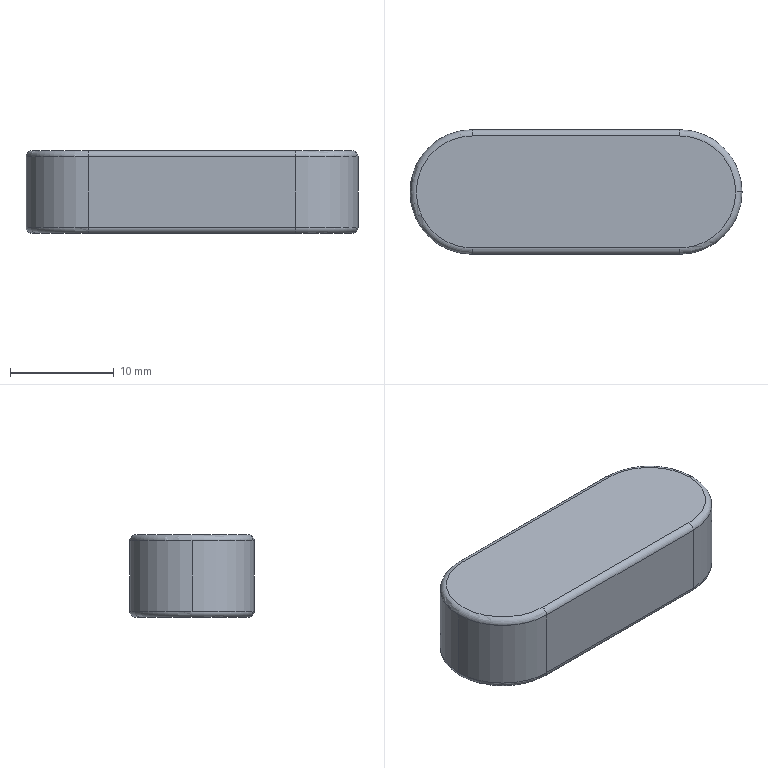Part | SolidWorks | features Extrusion 1, Fillet 1 | 1 solid | 17 faces | box 32 x 12 x 8 mm | volume 2813 mm3 | cylinder 7 | torus 6 | plane 4 | commonest cylinder face diameters 1.2 x4 12 x3
STEP:
#1=CARTESIAN_POINT('',(15.4,0.,0.));
#2=VERTEX_POINT('',#1);
#3=CARTESIAN_POINT('',(10.,-5.4,0.));
#4=VERTEX_POINT('',#3);
#5=CARTESIAN_POINT('',(10.,0.,0.));
#6=DIRECTION('',(0.,0.,-1.));
#7=DIRECTION('',(1.,0.,0.));
#8=AXIS2_PLACEMENT_3D('',#5,#6,#7);
#9=CIRCLE('',#8,5.4);
#10=EDGE_CURVE('',#2,#4,#9,.T.);
#11=ORIENTED_EDGE('',*,*,#10,.F.);
#12=CARTESIAN_POINT('',(16.,0.,0.6));
#13=VERTEX_POINT('',#12);
#14=CARTESIAN_POINT('',(15.4,0.,0.6));
#15=DIRECTION('',(0.,-1.,0.));
#16=DIRECTION('',(0.,0.,-1.));
#17=AXIS2_PLACEMENT_3D('',#14,#15,#16);
#18=CIRCLE('',#17,0.6);
#19=EDGE_CURVE('',#2,#13,#18,.T.);
#20=ORIENTED_EDGE('',*,*,#19,.T.);
#21=CARTESIAN_POINT('',(10.,-6.,0.6));
#22=VERTEX_POINT('',#21);
#23=CARTESIAN_POINT('',(10.,0.,0.6));
#24=DIRECTION('',(0.,0.,1.));
#25=DIRECTION('',(1.,0.,0.));
#26=AXIS2_PLACEMENT_3D('',#23,#24,#25);
#27=CIRCLE('',#26,6.);
#28=EDGE_CURVE('',#22,#13,#27,.T.);
#29=ORIENTED_EDGE('',*,*,#28,.F.);
#30=CARTESIAN_POINT('',(10.,-5.4,0.6));
#31=DIRECTION('',(1.,0.,0.));
#32=DIRECTION('',(0.,0.,-1.));
#33=AXIS2_PLACEMENT_3D('',#30,#31,#32);
#34=CIRCLE('',#33,0.6);
#35=EDGE_CURVE('',#22,#4,#34,.T.);
#36=ORIENTED_EDGE('',*,*,#35,.T.);
#37=EDGE_LOOP('',(#11,#20,#29,#36));
#38=FACE_OUTER_BOUND('',#37,.T.);
#39=CARTESIAN_POINT('',(10.,0.,0.6));
#40=DIRECTION('',(0.,0.,1.));
#41=DIRECTION('',(1.,0.,0.));
#42=AXIS2_PLACEMENT_3D('',#39,#40,#41);
#43=TOROIDAL_SURFACE('',#42,5.4,0.6);
#44=ADVANCED_FACE('',(#38),#43,.T.);
#45=CARTESIAN_POINT('',(16.,0.,7.4));
#46=VERTEX_POINT('',#45);
#47=CARTESIAN_POINT('',(10.,-6.,7.4));
#48=VERTEX_POINT('',#47);
#49=CARTESIAN_POINT('',(10.,0.,7.4));
#50=DIRECTION('',(0.,0.,-1.));
#51=DIRECTION('',(1.,0.,0.));
#52=AXIS2_PLACEMENT_3D('',#49,#50,#51);
#53=CIRCLE('',#52,6.);
#54=EDGE_CURVE('',#46,#48,#53,.T.);
#55=ORIENTED_EDGE('',*,*,#54,.F.);
#56=CARTESIAN_POINT('',(15.4,0.,8.));
#57=VERTEX_POINT('',#56);
#58=CARTESIAN_POINT('',(15.4,0.,7.4));
#59=DIRECTION('',(0.,-1.,0.));
#60=DIRECTION('',(0.,0.,-1.));
#61=AXIS2_PLACEMENT_3D('',#58,#59,#60);
#62=CIRCLE('',#61,0.6);
#63=EDGE_CURVE('',#46,#57,#62,.T.);
#64=ORIENTED_EDGE('',*,*,#63,.T.);
#65=CARTESIAN_POINT('',(10.,-5.4,8.));
#66=VERTEX_POINT('',#65);
#67=CARTESIAN_POINT('',(10.,0.,8.));
#68=DIRECTION('',(0.,0.,1.));
#69=DIRECTION('',(1.,0.,0.));
#70=AXIS2_PLACEMENT_3D('',#67,#68,#69);
#71=CIRCLE('',#70,5.4);
#72=EDGE_CURVE('',#66,#57,#71,.T.);
#73=ORIENTED_EDGE('',*,*,#72,.F.);
#74=CARTESIAN_POINT('',(10.,-5.4,7.4));
#75=DIRECTION('',(1.,0.,0.));
#76=DIRECTION('',(0.,0.,-1.));
#77=AXIS2_PLACEMENT_3D('',#74,#75,#76);
#78=CIRCLE('',#77,0.6);
#79=EDGE_CURVE('',#66,#48,#78,.T.);
#80=ORIENTED_EDGE('',*,*,#79,.T.);
#81=EDGE_LOOP('',(#55,#64,#73,#80));
#82=FACE_OUTER_BOUND('',#81,.T.);
#83=CARTESIAN_POINT('',(10.,0.,7.4));
#84=DIRECTION('',(0.,0.,1.));
#85=DIRECTION('',(1.,0.,0.));
#86=AXIS2_PLACEMENT_3D('',#83,#84,#85);
#87=TOROIDAL_SURFACE('',#86,5.4,0.6);
#88=ADVANCED_FACE('',(#82),#87,.T.);
#89=CARTESIAN_POINT('',(-10.,-6.,7.4));
#90=VERTEX_POINT('',#89);
#91=CARTESIAN_POINT('',(-16.,0.,7.4));
#92=VERTEX_POINT('',#91);
#93=CARTESIAN_POINT('',(-10.,0.,7.4));
#94=DIRECTION('',(0.,0.,-1.));
#95=DIRECTION('',(1.,0.,0.));
#96=AXIS2_PLACEMENT_3D('',#93,#94,#95);
#97=CIRCLE('',#96,6.);
#98=EDGE_CURVE('',#90,#92,#97,.T.);
#99=ORIENTED_EDGE('',*,*,#98,.T.);
#100=CARTESIAN_POINT('',(-16.,0.,0.6));
#101=VERTEX_POINT('',#100);
#102=CARTESIAN_POINT('',(-16.,0.,8.));
#103=DIRECTION('',(0.,0.,-1.));
#104=VECTOR('',#103,1000.);
#105=LINE('',#102,#104);
#106=EDGE_CURVE('',#92,#101,#105,.T.);
#107=ORIENTED_EDGE('',*,*,#106,.T.);
#108=CARTESIAN_POINT('',(-10.,-6.,0.6));
#109=VERTEX_POINT('',#108);
#110=CARTESIAN_POINT('',(-10.,0.,0.6));
#111=DIRECTION('',(0.,0.,1.));
#112=DIRECTION('',(1.,0.,0.));
#113=AXIS2_PLACEMENT_3D('',#110,#111,#112);
#114=CIRCLE('',#113,6.);
#115=EDGE_CURVE('',#101,#109,#114,.T.);
#116=ORIENTED_EDGE('',*,*,#115,.T.);
#117=CARTESIAN_POINT('',(-10.,-6.,8.));
#118=DIRECTION('',(0.,0.,-1.));
#119=VECTOR('',#118,1000.);
#120=LINE('',#117,#119);
#121=EDGE_CURVE('',#90,#109,#120,.T.);
#122=ORIENTED_EDGE('',*,*,#121,.F.);
#123=EDGE_LOOP('',(#99,#107,#116,#122));
#124=FACE_OUTER_BOUND('',#123,.T.);
#125=CARTESIAN_POINT('',(-10.,0.,8.));
#126=DIRECTION('',(0.,0.,-1.));
#127=DIRECTION('',(-1.,0.,0.));
#128=AXIS2_PLACEMENT_3D('',#125,#126,#127);
#129=CYLINDRICAL_SURFACE('',#128,6.);
#130=ADVANCED_FACE('',(#124),#129,.T.);
#131=ORIENTED_EDGE('',*,*,#106,.F.);
#132=CARTESIAN_POINT('',(-10.,6.,7.4));
#133=VERTEX_POINT('',#132);
#134=CARTESIAN_POINT('',(-10.,0.,7.4));
#135=DIRECTION('',(0.,0.,-1.));
#136=DIRECTION('',(1.,0.,0.));
#137=AXIS2_PLACEMENT_3D('',#134,#135,#136);
#138=CIRCLE('',#137,6.);
#139=EDGE_CURVE('',#92,#133,#138,.T.);
#140=ORIENTED_EDGE('',*,*,#139,.T.);
#141=CARTESIAN_POINT('',(-10.,6.,0.6));
#142=VERTEX_POINT('',#141);
#143=CARTESIAN_POINT('',(-10.,6.,8.));
#144=DIRECTION('',(0.,0.,-1.));
#145=VECTOR('',#144,1000.);
#146=LINE('',#143,#145);
#147=EDGE_CURVE('',#133,#142,#146,.T.);
#148=ORIENTED_EDGE('',*,*,#147,.T.);
#149=CARTESIAN_POINT('',(-10.,0.,0.6));
#150=DIRECTION('',(0.,0.,1.));
#151=DIRECTION('',(1.,0.,0.));
#152=AXIS2_PLACEMENT_3D('',#149,#150,#151);
#153=CIRCLE('',#152,6.);
#154=EDGE_CURVE('',#142,#101,#153,.T.);
#155=ORIENTED_EDGE('',*,*,#154,.T.);
#156=EDGE_LOOP('',(#131,#140,#148,#155));
#157=FACE_OUTER_BOUND('',#156,.T.);
#158=CARTESIAN_POINT('',(-10.,0.,8.));
#159=DIRECTION('',(0.,0.,-1.));
#160=DIRECTION('',(-1.,0.,0.));
#161=AXIS2_PLACEMENT_3D('',#158,#159,#160);
#162=CYLINDRICAL_SURFACE('',#161,6.);
#163=ADVANCED_FACE('',(#157),#162,.T.);
#164=CARTESIAN_POINT('',(10.,-6.,8.));
#165=DIRECTION('',(0.,0.,-1.));
#166=VECTOR('',#165,1000.);
#167=LINE('',#164,#166);
#168=EDGE_CURVE('',#48,#22,#167,.T.);
#169=ORIENTED_EDGE('',*,*,#168,.F.);
#170=CARTESIAN_POINT('',(-10.,-6.,7.4));
#171=DIRECTION('',(-1.,0.,0.));
#172=VECTOR('',#171,1000.);
#173=LINE('',#170,#172);
#174=EDGE_CURVE('',#48,#90,#173,.T.);
#175=ORIENTED_EDGE('',*,*,#174,.T.);
#176=ORIENTED_EDGE('',*,*,#121,.T.);
#177=CARTESIAN_POINT('',(-10.,-6.,0.6));
#178=DIRECTION('',(1.,0.,0.));
#179=VECTOR('',#178,1000.);
#180=LINE('',#177,#179);
#181=EDGE_CURVE('',#109,#22,#180,.T.);
#182=ORIENTED_EDGE('',*,*,#181,.T.);
#183=EDGE_LOOP('',(#169,#175,#176,#182));
#184=FACE_OUTER_BOUND('',#183,.T.);
#185=CARTESIAN_POINT('',(-10.,-6.,8.));
#186=DIRECTION('',(0.,1.,0.));
#187=DIRECTION('',(-1.,0.,0.));
#188=AXIS2_PLACEMENT_3D('',#185,#186,#187);
#189=PLANE('',#188);
#190=ADVANCED_FACE('',(#184),#189,.F.);
#191=CARTESIAN_POINT('',(10.,6.,7.4));
#192=VERTEX_POINT('',#191);
#193=CARTESIAN_POINT('',(10.,6.,0.6));
#194=VERTEX_POINT('',#193);
#195=CARTESIAN_POINT('',(10.,6.,8.));
#196=DIRECTION('',(0.,0.,-1.));
#197=VECTOR('',#196,1000.);
#198=LINE('',#195,#197);
#199=EDGE_CURVE('',#192,#194,#198,.T.);
#200=ORIENTED_EDGE('',*,*,#199,.F.);
#201=CARTESIAN_POINT('',(10.,0.,7.4));
#202=DIRECTION('',(0.,0.,-1.));
#203=DIRECTION('',(1.,0.,0.));
#204=AXIS2_PLACEMENT_3D('',#201,#202,#203);
#205=CIRCLE('',#204,6.);
#206=EDGE_CURVE('',#192,#46,#205,.T.);
#207=ORIENTED_EDGE('',*,*,#206,.T.);
#208=ORIENTED_EDGE('',*,*,#54,.T.);
#209=ORIENTED_EDGE('',*,*,#168,.T.);
#210=ORIENTED_EDGE('',*,*,#28,.T.);
#211=CARTESIAN_POINT('',(10.,0.,0.6));
#212=DIRECTION('',(0.,0.,1.));
#213=DIRECTION('',(1.,0.,0.));
#214=AXIS2_PLACEMENT_3D('',#211,#212,#213);
#215=CIRCLE('',#214,6.);
#216=EDGE_CURVE('',#13,#194,#215,.T.);
#217=ORIENTED_EDGE('',*,*,#216,.T.);
#218=EDGE_LOOP('',(#200,#207,#208,#209,#210,#217));
#219=FACE_OUTER_BOUND('',#218,.T.);
#220=CARTESIAN_POINT('',(10.,0.,8.));
#221=DIRECTION('',(0.,0.,-1.));
#222=DIRECTION('',(-1.,0.,0.));
#223=AXIS2_PLACEMENT_3D('',#220,#221,#222);
#224=CYLINDRICAL_SURFACE('',#223,6.);
#225=ADVANCED_FACE('',(#219),#224,.T.);
#226=ORIENTED_EDGE('',*,*,#147,.F.);
#227=CARTESIAN_POINT('',(10.,6.,7.4));
#228=DIRECTION('',(1.,0.,0.));
#229=VECTOR('',#228,1000.);
#230=LINE('',#227,#229);
#231=EDGE_CURVE('',#133,#192,#230,.T.);
#232=ORIENTED_EDGE('',*,*,#231,.T.);
#233=ORIENTED_EDGE('',*,*,#199,.T.);
#234=CARTESIAN_POINT('',(-10.,6.,0.6));
#235=DIRECTION('',(-1.,0.,0.));
#236=VECTOR('',#235,1000.);
#237=LINE('',#234,#236);
#238=EDGE_CURVE('',#194,#142,#237,.T.);
#239=ORIENTED_EDGE('',*,*,#238,.T.);
#240=EDGE_LOOP('',(#226,#232,#233,#239));
#241=FACE_OUTER_BOUND('',#240,.T.);
#242=CARTESIAN_POINT('',(-10.,6.,8.));
#243=DIRECTION('',(0.,-1.,0.));
#244=DIRECTION('',(1.,0.,0.));
#245=AXIS2_PLACEMENT_3D('',#242,#243,#244);
#246=PLANE('',#245);
#247=ADVANCED_FACE('',(#241),#246,.F.);
#248=CARTESIAN_POINT('',(-10.,-5.4,8.));
#249=VERTEX_POINT('',#248);
#250=CARTESIAN_POINT('',(10.,-5.4,8.));
#251=DIRECTION('',(1.,0.,0.));
#252=VECTOR('',#251,1000.);
#253=LINE('',#250,#252);
#254=EDGE_CURVE('',#249,#66,#253,.T.);
#255=ORIENTED_EDGE('',*,*,#254,.T.);
#256=ORIENTED_EDGE('',*,*,#72,.T.);
#257=CARTESIAN_POINT('',(10.,5.4,8.));
#258=VERTEX_POINT('',#257);
#259=CARTESIAN_POINT('',(10.,0.,8.));
#260=DIRECTION('',(0.,0.,1.));
#261=DIRECTION('',(1.,0.,0.));
#262=AXIS2_PLACEMENT_3D('',#259,#260,#261);
#263=CIRCLE('',#262,5.4);
#264=EDGE_CURVE('',#57,#258,#263,.T.);
#265=ORIENTED_EDGE('',*,*,#264,.T.);
#266=CARTESIAN_POINT('',(-10.,5.4,8.));
#267=VERTEX_POINT('',#266);
#268=CARTESIAN_POINT('',(-10.,5.4,8.));
#269=DIRECTION('',(-1.,0.,0.));
#270=VECTOR('',#269,1000.);
#271=LINE('',#268,#270);
#272=EDGE_CURVE('',#258,#267,#271,.T.);
#273=ORIENTED_EDGE('',*,*,#272,.T.);
#274=CARTESIAN_POINT('',(-10.,0.,8.));
#275=DIRECTION('',(0.,0.,1.));
#276=DIRECTION('',(1.,0.,0.));
#277=AXIS2_PLACEMENT_3D('',#274,#275,#276);
#278=CIRCLE('',#277,5.4);
#279=EDGE_CURVE('',#267,#249,#278,.T.);
#280=ORIENTED_EDGE('',*,*,#279,.T.);
#281=EDGE_LOOP('',(#255,#256,#265,#273,#280));
#282=FACE_OUTER_BOUND('',#281,.T.);
#283=CARTESIAN_POINT('',(-10.,0.,8.));
#284=DIRECTION('',(0.,0.,1.));
#285=DIRECTION('',(1.,0.,0.));
#286=AXIS2_PLACEMENT_3D('',#283,#284,#285);
#287=PLANE('',#286);
#288=ADVANCED_FACE('',(#282),#287,.T.);
#289=CARTESIAN_POINT('',(-10.,5.4,0.));
#290=VERTEX_POINT('',#289);
#291=CARTESIAN_POINT('',(10.,5.4,0.));
#292=VERTEX_POINT('',#291);
#293=CARTESIAN_POINT('',(-10.,5.4,0.));
#294=DIRECTION('',(1.,0.,0.));
#295=VECTOR('',#294,1000.);
#296=LINE('',#293,#295);
#297=EDGE_CURVE('',#290,#292,#296,.T.);
#298=ORIENTED_EDGE('',*,*,#297,.T.);
#299=CARTESIAN_POINT('',(10.,0.,0.));
#300=DIRECTION('',(0.,0.,-1.));
#301=DIRECTION('',(1.,0.,0.));
#302=AXIS2_PLACEMENT_3D('',#299,#300,#301);
#303=CIRCLE('',#302,5.4);
#304=EDGE_CURVE('',#292,#2,#303,.T.);
#305=ORIENTED_EDGE('',*,*,#304,.T.);
#306=ORIENTED_EDGE('',*,*,#10,.T.);
#307=CARTESIAN_POINT('',(-10.,-5.4,0.));
#308=VERTEX_POINT('',#307);
#309=CARTESIAN_POINT('',(-10.,-5.4,0.));
#310=DIRECTION('',(-1.,0.,0.));
#311=VECTOR('',#310,1000.);
#312=LINE('',#309,#311);
#313=EDGE_CURVE('',#4,#308,#312,.T.);
#314=ORIENTED_EDGE('',*,*,#313,.T.);
#315=CARTESIAN_POINT('',(-10.,0.,0.));
#316=DIRECTION('',(0.,0.,-1.));
#317=DIRECTION('',(1.,0.,0.));
#318=AXIS2_PLACEMENT_3D('',#315,#316,#317);
#319=CIRCLE('',#318,5.4);
#320=EDGE_CURVE('',#308,#290,#319,.T.);
#321=ORIENTED_EDGE('',*,*,#320,.T.);
#322=EDGE_LOOP('',(#298,#305,#306,#314,#321));
#323=FACE_OUTER_BOUND('',#322,.T.);
#324=CARTESIAN_POINT('',(-10.,0.,0.));
#325=DIRECTION('',(0.,0.,1.));
#326=DIRECTION('',(1.,0.,0.));
#327=AXIS2_PLACEMENT_3D('',#324,#325,#326);
#328=PLANE('',#327);
#329=ADVANCED_FACE('',(#323),#328,.F.);
#330=CARTESIAN_POINT('',(-10.,5.4,7.4));
#331=DIRECTION('',(1.,0.,0.));
#332=DIRECTION('',(0.,0.,-1.));
#333=AXIS2_PLACEMENT_3D('',#330,#331,#332);
#334=CIRCLE('',#333,0.6);
#335=EDGE_CURVE('',#133,#267,#334,.T.);
#336=ORIENTED_EDGE('',*,*,#335,.F.);
#337=ORIENTED_EDGE('',*,*,#139,.F.);
#338=ORIENTED_EDGE('',*,*,#98,.F.);
#339=CARTESIAN_POINT('',(-10.,-5.4,7.4));
#340=DIRECTION('',(1.,0.,0.));
#341=DIRECTION('',(0.,0.,-1.));
#342=AXIS2_PLACEMENT_3D('',#339,#340,#341);
#343=CIRCLE('',#342,0.6);
#344=EDGE_CURVE('',#249,#90,#343,.T.);
#345=ORIENTED_EDGE('',*,*,#344,.F.);
#346=ORIENTED_EDGE('',*,*,#279,.F.);
#347=EDGE_LOOP('',(#336,#337,#338,#345,#346));
#348=FACE_OUTER_BOUND('',#347,.T.);
#349=CARTESIAN_POINT('',(-10.,0.,7.4));
#350=DIRECTION('',(0.,0.,1.));
#351=DIRECTION('',(1.,0.,0.));
#352=AXIS2_PLACEMENT_3D('',#349,#350,#351);
#353=TOROIDAL_SURFACE('',#352,5.4,0.6);
#354=ADVANCED_FACE('',(#348),#353,.T.);
#355=ORIENTED_EDGE('',*,*,#344,.T.);
#356=ORIENTED_EDGE('',*,*,#174,.F.);
#357=ORIENTED_EDGE('',*,*,#79,.F.);
#358=ORIENTED_EDGE('',*,*,#254,.F.);
#359=EDGE_LOOP('',(#355,#356,#357,#358));
#360=FACE_OUTER_BOUND('',#359,.T.);
#361=CARTESIAN_POINT('',(-10.,-5.4,7.4));
#362=DIRECTION('',(-1.,0.,0.));
#363=DIRECTION('',(0.,-1.,0.));
#364=AXIS2_PLACEMENT_3D('',#361,#362,#363);
#365=CYLINDRICAL_SURFACE('',#364,0.6);
#366=ADVANCED_FACE('',(#360),#365,.T.);
#367=ORIENTED_EDGE('',*,*,#335,.T.);
#368=ORIENTED_EDGE('',*,*,#272,.F.);
#369=CARTESIAN_POINT('',(10.,5.4,7.4));
#370=DIRECTION('',(1.,0.,0.));
#371=DIRECTION('',(0.,0.,-1.));
#372=AXIS2_PLACEMENT_3D('',#369,#370,#371);
#373=CIRCLE('',#372,0.6);
#374=EDGE_CURVE('',#192,#258,#373,.T.);
#375=ORIENTED_EDGE('',*,*,#374,.F.);
#376=ORIENTED_EDGE('',*,*,#231,.F.);
#377=EDGE_LOOP('',(#367,#368,#375,#376));
#378=FACE_OUTER_BOUND('',#377,.T.);
#379=CARTESIAN_POINT('',(-10.,5.4,7.4));
#380=DIRECTION('',(1.,0.,0.));
#381=DIRECTION('',(0.,1.,0.));
#382=AXIS2_PLACEMENT_3D('',#379,#380,#381);
#383=CYLINDRICAL_SURFACE('',#382,0.6);
#384=ADVANCED_FACE('',(#378),#383,.T.);
#385=ORIENTED_EDGE('',*,*,#63,.F.);
#386=ORIENTED_EDGE('',*,*,#206,.F.);
#387=ORIENTED_EDGE('',*,*,#374,.T.);
#388=ORIENTED_EDGE('',*,*,#264,.F.);
#389=EDGE_LOOP('',(#385,#386,#387,#388));
#390=FACE_OUTER_BOUND('',#389,.T.);
#391=CARTESIAN_POINT('',(10.,0.,7.4));
#392=DIRECTION('',(0.,0.,1.));
#393=DIRECTION('',(1.,0.,0.));
#394=AXIS2_PLACEMENT_3D('',#391,#392,#393);
#395=TOROIDAL_SURFACE('',#394,5.4,0.6);
#396=ADVANCED_FACE('',(#390),#395,.T.);
#397=CARTESIAN_POINT('',(-10.,5.4,0.6));
#398=DIRECTION('',(1.,0.,0.));
#399=DIRECTION('',(0.,0.,-1.));
#400=AXIS2_PLACEMENT_3D('',#397,#398,#399);
#401=CIRCLE('',#400,0.6);
#402=EDGE_CURVE('',#290,#142,#401,.T.);
#403=ORIENTED_EDGE('',*,*,#402,.F.);
#404=ORIENTED_EDGE('',*,*,#320,.F.);
#405=CARTESIAN_POINT('',(-10.,-5.4,0.6));
#406=DIRECTION('',(1.,0.,0.));
#407=DIRECTION('',(0.,0.,-1.));
#408=AXIS2_PLACEMENT_3D('',#405,#406,#407);
#409=CIRCLE('',#408,0.6);
#410=EDGE_CURVE('',#109,#308,#409,.T.);
#411=ORIENTED_EDGE('',*,*,#410,.F.);
#412=ORIENTED_EDGE('',*,*,#115,.F.);
#413=ORIENTED_EDGE('',*,*,#154,.F.);
#414=EDGE_LOOP('',(#403,#404,#411,#412,#413));
#415=FACE_OUTER_BOUND('',#414,.T.);
#416=CARTESIAN_POINT('',(-10.,0.,0.6));
#417=DIRECTION('',(0.,0.,1.));
#418=DIRECTION('',(1.,0.,0.));
#419=AXIS2_PLACEMENT_3D('',#416,#417,#418);
#420=TOROIDAL_SURFACE('',#419,5.4,0.6);
#421=ADVANCED_FACE('',(#415),#420,.T.);
#422=ORIENTED_EDGE('',*,*,#410,.T.);
#423=ORIENTED_EDGE('',*,*,#313,.F.);
#424=ORIENTED_EDGE('',*,*,#35,.F.);
#425=ORIENTED_EDGE('',*,*,#181,.F.);
#426=EDGE_LOOP('',(#422,#423,#424,#425));
#427=FACE_OUTER_BOUND('',#426,.T.);
#428=CARTESIAN_POINT('',(-10.,-5.4,0.6));
#429=DIRECTION('',(1.,0.,0.));
#430=DIRECTION('',(0.,1.,0.));
#431=AXIS2_PLACEMENT_3D('',#428,#429,#430);
#432=CYLINDRICAL_SURFACE('',#431,0.6);
#433=ADVANCED_FACE('',(#427),#432,.T.);
#434=ORIENTED_EDGE('',*,*,#402,.T.);
#435=ORIENTED_EDGE('',*,*,#238,.F.);
#436=CARTESIAN_POINT('',(10.,5.4,0.6));
#437=DIRECTION('',(1.,0.,0.));
#438=DIRECTION('',(0.,0.,-1.));
#439=AXIS2_PLACEMENT_3D('',#436,#437,#438);
#440=CIRCLE('',#439,0.6);
#441=EDGE_CURVE('',#292,#194,#440,.T.);
#442=ORIENTED_EDGE('',*,*,#441,.F.);
#443=ORIENTED_EDGE('',*,*,#297,.F.);
#444=EDGE_LOOP('',(#434,#435,#442,#443));
#445=FACE_OUTER_BOUND('',#444,.T.);
#446=CARTESIAN_POINT('',(-10.,5.4,0.6));
#447=DIRECTION('',(-1.,0.,0.));
#448=DIRECTION('',(0.,-1.,0.));
#449=AXIS2_PLACEMENT_3D('',#446,#447,#448);
#450=CYLINDRICAL_SURFACE('',#449,0.6);
#451=ADVANCED_FACE('',(#445),#450,.T.);
#452=ORIENTED_EDGE('',*,*,#19,.F.);
#453=ORIENTED_EDGE('',*,*,#304,.F.);
#454=ORIENTED_EDGE('',*,*,#441,.T.);
#455=ORIENTED_EDGE('',*,*,#216,.F.);
#456=EDGE_LOOP('',(#452,#453,#454,#455));
#457=FACE_OUTER_BOUND('',#456,.T.);
#458=CARTESIAN_POINT('',(10.,0.,0.6));
#459=DIRECTION('',(0.,0.,1.));
#460=DIRECTION('',(1.,0.,0.));
#461=AXIS2_PLACEMENT_3D('',#458,#459,#460);
#462=TOROIDAL_SURFACE('',#461,5.4,0.6);
#463=ADVANCED_FACE('',(#457),#462,.T.);
#464=CLOSED_SHELL('',(#44,#88,#130,#163,#190,#225,#247,#288,#329,#354,#366,#384,#396,#421,#433,#451,#463));
#465=MANIFOLD_SOLID_BREP('',#464);
#466=CARTESIAN_POINT('',(0.,0.,0.));
#467=DIRECTION('',(0.,0.,1.));
#468=DIRECTION('',(1.,0.,0.));
#469=AXIS2_PLACEMENT_3D('',#466,#467,#468);
#470=(LENGTH_UNIT()NAMED_UNIT(*)SI_UNIT(.MILLI.,.METRE.));
#471=UNCERTAINTY_MEASURE_WITH_UNIT(LENGTH_MEASURE(0.00001),#470,'','');
#472=(NAMED_UNIT(*)PLANE_ANGLE_UNIT()SI_UNIT($,.RADIAN.));
#473=(NAMED_UNIT(*)SI_UNIT($,.STERADIAN.)SOLID_ANGLE_UNIT());
#474=(GEOMETRIC_REPRESENTATION_CONTEXT(3)GLOBAL_UNCERTAINTY_ASSIGNED_CONTEXT((#471))GLOBAL_UNIT_ASSIGNED_CONTEXT((#470,#472,#473))REPRESENTATION_CONTEXT('',''));
#475=ADVANCED_BREP_SHAPE_REPRESENTATION('',(#465,#469),#474);